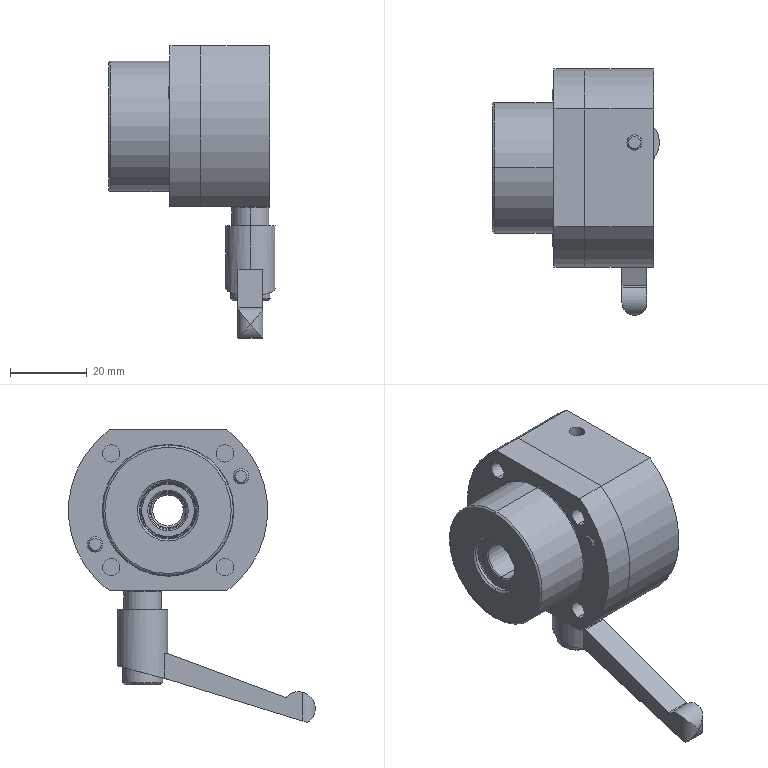Part | STEP file | 001-003-LHF08-Q10, | 8 solids | 503 faces | box 43.5 x 64.4 x 76.26 mm | volume 63450 mm3 | cylinder 163 | cone 136 | plane 110 | torus 94 | commonest cylinder face diameters 8 x14 4.5 x12 2.1 x8 3.242 x8 4 x8 13.3 x8